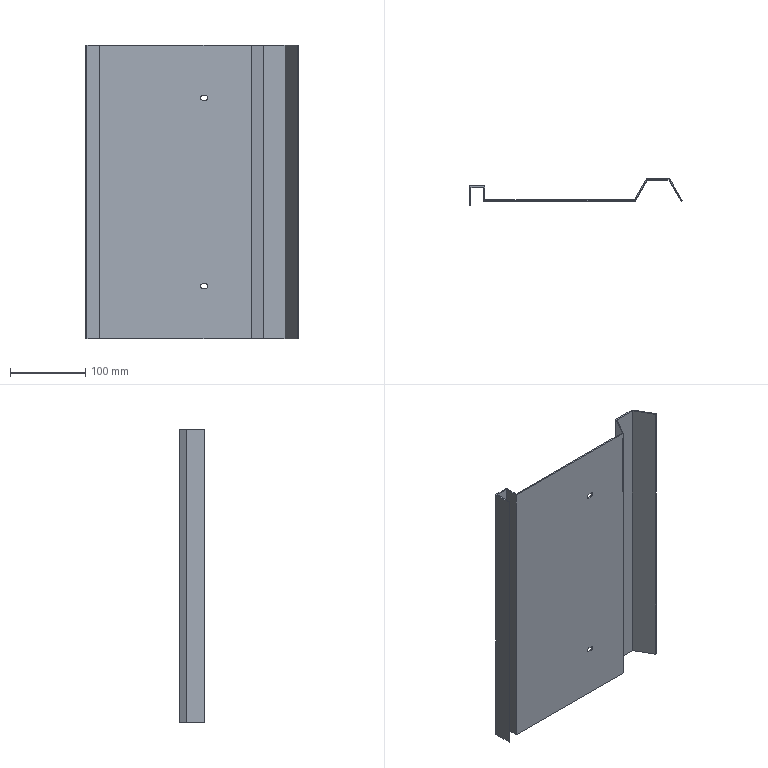Part | STEP file | 1 solid | 26 faces | box 281.999 x 34.5 x 390 mm | volume 208043 mm3 | plane 22 | cylinder 4 | commonest cylinder face diameters 6 x4